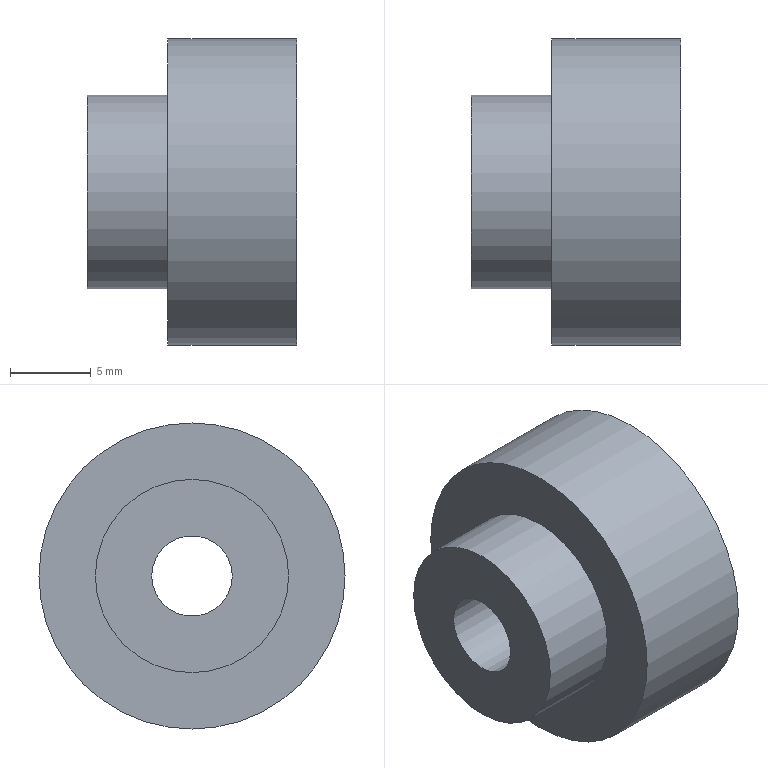Part | STEP file | 1-46.3 | 1 solid | 6 faces | box 13 x 19 x 19 mm | volume 2578 mm3 | plane 3 | cylinder 3 | commonest cylinder face diameters 5 x1 12 x1 19 x1
STEP:
#1=CARTESIAN_POINT('',(0.,0.,0.));
#2=DIRECTION('',(0.,0.,1.));
#3=DIRECTION('',(1.,0.,0.));
#4=AXIS2_PLACEMENT_3D('',#1,#2,#3);
#5=CARTESIAN_POINT('',(-5.,6.,0.));
#6=VERTEX_POINT('',#5);
#7=CARTESIAN_POINT('',(-5.,0.,0.));
#8=DIRECTION('',(1.,0.,0.));
#9=DIRECTION('',(0.,1.,0.));
#10=AXIS2_PLACEMENT_3D('',#7,#8,#9);
#11=CIRCLE('',#10,6.);
#12=CARTESIAN_POINT('',(-5.,-1.608,0.));
#13=DIRECTION('',(1.,0.,0.));
#14=DIRECTION('',(0.,0.,-1.));
#15=AXIS2_PLACEMENT_3D('',#12,#13,#14);
#16=PLANE('',#15);
#17=CARTESIAN_POINT('',(0.,1.608));
#18=DIRECTION('',(0.,1.));
#19=AXIS2_PLACEMENT_2D('',#17,#18);
#20=CIRCLE('',#19,6.);
#21=(GEOMETRIC_REPRESENTATION_CONTEXT(2)PARAMETRIC_REPRESENTATION_CONTEXT()REPRESENTATION_CONTEXT('',''));
#22=DEFINITIONAL_REPRESENTATION('',(#20),#21);
#23=PCURVE('',#16,#22);
#24=CARTESIAN_POINT('',(0.,0.,0.));
#25=DIRECTION('',(-1.,0.,0.));
#26=DIRECTION('',(0.,1.,0.));
#27=AXIS2_PLACEMENT_3D('',#24,#25,#26);
#28=CYLINDRICAL_SURFACE('',#27,6.);
#29=CARTESIAN_POINT('',(6.283,5.));
#30=DIRECTION('',(-1.,0.));
#31=VECTOR('',#30,1.);
#32=LINE('',#29,#31);
#33=(GEOMETRIC_REPRESENTATION_CONTEXT(2)PARAMETRIC_REPRESENTATION_CONTEXT()REPRESENTATION_CONTEXT('',''));
#34=DEFINITIONAL_REPRESENTATION('',(#32),#33);
#35=PCURVE('',#28,#34);
#36=SURFACE_CURVE('',#11,(#23,#35),.PCURVE_S1.);
#37=EDGE_CURVE('',#6,#6,#36,.T.);
#38=ORIENTED_EDGE('',*,*,#37,.T.);
#39=EDGE_LOOP('',(#38));
#40=FACE_BOUND('',#39,.F.);
#41=CARTESIAN_POINT('',(-5.,2.5,0.));
#42=VERTEX_POINT('',#41);
#43=CARTESIAN_POINT('',(-5.,0.,0.));
#44=DIRECTION('',(-1.,0.,0.));
#45=DIRECTION('',(0.,1.,0.));
#46=AXIS2_PLACEMENT_3D('',#43,#44,#45);
#47=CIRCLE('',#46,2.5);
#48=CARTESIAN_POINT('',(0.,4.108));
#49=CARTESIAN_POINT('',(4.33,4.108));
#50=CARTESIAN_POINT('',(2.165,0.3577));
#51=CARTESIAN_POINT('',(0.,-3.392));
#52=CARTESIAN_POINT('',(-2.165,0.3577));
#53=CARTESIAN_POINT('',(-4.33,4.108));
#54=CARTESIAN_POINT('',(0.,4.108));
#55=(BOUNDED_CURVE()B_SPLINE_CURVE(2,(#48,#49,#50,#51,#52,#53,#54),.UNSPECIFIED.,.T.,.F.)B_SPLINE_CURVE_WITH_KNOTS((1,2,2,2,2,1),(-2.094,0.,2.094,4.189,6.283,8.378),.UNSPECIFIED.)CURVE()GEOMETRIC_REPRESENTATION_ITEM()RATIONAL_B_SPLINE_CURVE((1.,0.5,1.,0.5,1.,0.5,1.))REPRESENTATION_ITEM(''));
#56=(GEOMETRIC_REPRESENTATION_CONTEXT(2)PARAMETRIC_REPRESENTATION_CONTEXT()REPRESENTATION_CONTEXT('',''));
#57=DEFINITIONAL_REPRESENTATION('',(#55),#56);
#58=PCURVE('',#16,#57);
#59=CARTESIAN_POINT('',(8.,0.,0.));
#60=DIRECTION('',(-1.,0.,0.));
#61=DIRECTION('',(0.,1.,0.));
#62=AXIS2_PLACEMENT_3D('',#59,#60,#61);
#63=CYLINDRICAL_SURFACE('',#62,2.5);
#64=CARTESIAN_POINT('',(0.,13.));
#65=DIRECTION('',(1.,0.));
#66=VECTOR('',#65,1.);
#67=LINE('',#64,#66);
#68=(GEOMETRIC_REPRESENTATION_CONTEXT(2)PARAMETRIC_REPRESENTATION_CONTEXT()REPRESENTATION_CONTEXT('',''));
#69=DEFINITIONAL_REPRESENTATION('',(#67),#68);
#70=PCURVE('',#63,#69);
#71=SURFACE_CURVE('',#47,(#58,#70),.PCURVE_S1.);
#72=EDGE_CURVE('',#42,#42,#71,.T.);
#73=ORIENTED_EDGE('',*,*,#72,.T.);
#74=EDGE_LOOP('',(#73));
#75=FACE_BOUND('',#74,.F.);
#76=ADVANCED_FACE('',(#40,#75),#16,.F.);
#77=CARTESIAN_POINT('',(0.,6.,0.));
#78=VERTEX_POINT('',#77);
#79=CARTESIAN_POINT('',(0.,6.,0.));
#80=DIRECTION('',(-1.,0.,0.));
#81=VECTOR('',#80,1.);
#82=LINE('',#79,#81);
#83=CARTESIAN_POINT('',(6.283,0.));
#84=DIRECTION('',(0.,1.));
#85=VECTOR('',#84,1.);
#86=LINE('',#83,#85);
#87=(GEOMETRIC_REPRESENTATION_CONTEXT(2)PARAMETRIC_REPRESENTATION_CONTEXT()REPRESENTATION_CONTEXT('',''));
#88=DEFINITIONAL_REPRESENTATION('',(#86),#87);
#89=PCURVE('',#28,#88);
#90=CARTESIAN_POINT('',(0.,0.));
#91=DIRECTION('',(0.,1.));
#92=VECTOR('',#91,1.);
#93=LINE('',#90,#92);
#94=(GEOMETRIC_REPRESENTATION_CONTEXT(2)PARAMETRIC_REPRESENTATION_CONTEXT()REPRESENTATION_CONTEXT('',''));
#95=DEFINITIONAL_REPRESENTATION('',(#93),#94);
#96=PCURVE('',#28,#95);
#97=SEAM_CURVE('',#82,(#89,#96),.PCURVE_S1.);
#98=EDGE_CURVE('',#78,#6,#97,.T.);
#99=ORIENTED_EDGE('',*,*,#98,.T.);
#100=ORIENTED_EDGE('',*,*,#37,.T.);
#101=ORIENTED_EDGE('',*,*,#98,.F.);
#102=CARTESIAN_POINT('',(0.,0.,0.));
#103=DIRECTION('',(1.,0.,0.));
#104=DIRECTION('',(0.,1.,0.));
#105=AXIS2_PLACEMENT_3D('',#102,#103,#104);
#106=CIRCLE('',#105,6.);
#107=CARTESIAN_POINT('',(6.283,0.));
#108=DIRECTION('',(-1.,0.));
#109=VECTOR('',#108,1.);
#110=LINE('',#107,#109);
#111=(GEOMETRIC_REPRESENTATION_CONTEXT(2)PARAMETRIC_REPRESENTATION_CONTEXT()REPRESENTATION_CONTEXT('',''));
#112=DEFINITIONAL_REPRESENTATION('',(#110),#111);
#113=PCURVE('',#28,#112);
#114=CARTESIAN_POINT('',(0.,-2.546,0.));
#115=DIRECTION('',(1.,0.,0.));
#116=DIRECTION('',(0.,0.,-1.));
#117=AXIS2_PLACEMENT_3D('',#114,#115,#116);
#118=PLANE('',#117);
#119=CARTESIAN_POINT('',(0.,2.546));
#120=DIRECTION('',(0.,1.));
#121=AXIS2_PLACEMENT_2D('',#119,#120);
#122=CIRCLE('',#121,6.);
#123=(GEOMETRIC_REPRESENTATION_CONTEXT(2)PARAMETRIC_REPRESENTATION_CONTEXT()REPRESENTATION_CONTEXT('',''));
#124=DEFINITIONAL_REPRESENTATION('',(#122),#123);
#125=PCURVE('',#118,#124);
#126=SURFACE_CURVE('',#106,(#113,#125),.PCURVE_S1.);
#127=EDGE_CURVE('',#78,#78,#126,.T.);
#128=ORIENTED_EDGE('',*,*,#127,.F.);
#129=EDGE_LOOP('',(#99,#100,#101,#128));
#130=FACE_BOUND('',#129,.T.);
#131=ADVANCED_FACE('',(#130),#28,.T.);
#132=ORIENTED_EDGE('',*,*,#72,.F.);
#133=CARTESIAN_POINT('',(8.,2.5,0.));
#134=VERTEX_POINT('',#133);
#135=CARTESIAN_POINT('',(-5.,2.5,0.));
#136=DIRECTION('',(1.,0.,0.));
#137=VECTOR('',#136,1.);
#138=LINE('',#135,#137);
#139=CARTESIAN_POINT('',(0.,13.));
#140=DIRECTION('',(0.,-1.));
#141=VECTOR('',#140,1.);
#142=LINE('',#139,#141);
#143=(GEOMETRIC_REPRESENTATION_CONTEXT(2)PARAMETRIC_REPRESENTATION_CONTEXT()REPRESENTATION_CONTEXT('',''));
#144=DEFINITIONAL_REPRESENTATION('',(#142),#143);
#145=PCURVE('',#63,#144);
#146=CARTESIAN_POINT('',(6.283,13.));
#147=DIRECTION('',(0.,-1.));
#148=VECTOR('',#147,1.);
#149=LINE('',#146,#148);
#150=(GEOMETRIC_REPRESENTATION_CONTEXT(2)PARAMETRIC_REPRESENTATION_CONTEXT()REPRESENTATION_CONTEXT('',''));
#151=DEFINITIONAL_REPRESENTATION('',(#149),#150);
#152=PCURVE('',#63,#151);
#153=SEAM_CURVE('',#138,(#145,#152),.PCURVE_S1.);
#154=EDGE_CURVE('',#42,#134,#153,.T.);
#155=ORIENTED_EDGE('',*,*,#154,.T.);
#156=CARTESIAN_POINT('',(8.,0.,0.));
#157=DIRECTION('',(-1.,0.,0.));
#158=DIRECTION('',(0.,1.,0.));
#159=AXIS2_PLACEMENT_3D('',#156,#157,#158);
#160=CIRCLE('',#159,2.5);
#161=CARTESIAN_POINT('',(0.,0.));
#162=DIRECTION('',(1.,0.));
#163=VECTOR('',#162,1.);
#164=LINE('',#161,#163);
#165=(GEOMETRIC_REPRESENTATION_CONTEXT(2)PARAMETRIC_REPRESENTATION_CONTEXT()REPRESENTATION_CONTEXT('',''));
#166=DEFINITIONAL_REPRESENTATION('',(#164),#165);
#167=PCURVE('',#63,#166);
#168=CARTESIAN_POINT('',(8.,-2.546,0.));
#169=DIRECTION('',(1.,0.,0.));
#170=DIRECTION('',(0.,0.,-1.));
#171=AXIS2_PLACEMENT_3D('',#168,#169,#170);
#172=PLANE('',#171);
#173=CARTESIAN_POINT('',(0.,5.046));
#174=CARTESIAN_POINT('',(4.33,5.046));
#175=CARTESIAN_POINT('',(2.165,1.296));
#176=CARTESIAN_POINT('',(0.,-2.454));
#177=CARTESIAN_POINT('',(-2.165,1.296));
#178=CARTESIAN_POINT('',(-4.33,5.046));
#179=CARTESIAN_POINT('',(0.,5.046));
#180=(BOUNDED_CURVE()B_SPLINE_CURVE(2,(#173,#174,#175,#176,#177,#178,#179),.UNSPECIFIED.,.T.,.F.)B_SPLINE_CURVE_WITH_KNOTS((1,2,2,2,2,1),(-2.094,0.,2.094,4.189,6.283,8.378),.UNSPECIFIED.)CURVE()GEOMETRIC_REPRESENTATION_ITEM()RATIONAL_B_SPLINE_CURVE((1.,0.5,1.,0.5,1.,0.5,1.))REPRESENTATION_ITEM(''));
#181=(GEOMETRIC_REPRESENTATION_CONTEXT(2)PARAMETRIC_REPRESENTATION_CONTEXT()REPRESENTATION_CONTEXT('',''));
#182=DEFINITIONAL_REPRESENTATION('',(#180),#181);
#183=PCURVE('',#172,#182);
#184=SURFACE_CURVE('',#160,(#167,#183),.PCURVE_S1.);
#185=EDGE_CURVE('',#134,#134,#184,.T.);
#186=ORIENTED_EDGE('',*,*,#185,.T.);
#187=ORIENTED_EDGE('',*,*,#154,.F.);
#188=EDGE_LOOP('',(#132,#155,#186,#187));
#189=FACE_BOUND('',#188,.F.);
#190=ADVANCED_FACE('',(#189),#63,.F.);
#191=CARTESIAN_POINT('',(0.,9.5,0.));
#192=VERTEX_POINT('',#191);
#193=CARTESIAN_POINT('',(0.,0.,0.));
#194=DIRECTION('',(1.,0.,0.));
#195=DIRECTION('',(0.,1.,0.));
#196=AXIS2_PLACEMENT_3D('',#193,#194,#195);
#197=CIRCLE('',#196,9.5);
#198=CARTESIAN_POINT('',(0.,2.546));
#199=DIRECTION('',(0.,1.));
#200=AXIS2_PLACEMENT_2D('',#198,#199);
#201=CIRCLE('',#200,9.5);
#202=(GEOMETRIC_REPRESENTATION_CONTEXT(2)PARAMETRIC_REPRESENTATION_CONTEXT()REPRESENTATION_CONTEXT('',''));
#203=DEFINITIONAL_REPRESENTATION('',(#201),#202);
#204=PCURVE('',#118,#203);
#205=CARTESIAN_POINT('',(0.,0.,0.));
#206=DIRECTION('',(1.,0.,0.));
#207=DIRECTION('',(0.,1.,0.));
#208=AXIS2_PLACEMENT_3D('',#205,#206,#207);
#209=CYLINDRICAL_SURFACE('',#208,9.5);
#210=CARTESIAN_POINT('',(0.,0.));
#211=DIRECTION('',(1.,0.));
#212=VECTOR('',#211,1.);
#213=LINE('',#210,#212);
#214=(GEOMETRIC_REPRESENTATION_CONTEXT(2)PARAMETRIC_REPRESENTATION_CONTEXT()REPRESENTATION_CONTEXT('',''));
#215=DEFINITIONAL_REPRESENTATION('',(#213),#214);
#216=PCURVE('',#209,#215);
#217=SURFACE_CURVE('',#197,(#204,#216),.PCURVE_S1.);
#218=EDGE_CURVE('',#192,#192,#217,.T.);
#219=ORIENTED_EDGE('',*,*,#218,.T.);
#220=EDGE_LOOP('',(#219));
#221=FACE_BOUND('',#220,.F.);
#222=ORIENTED_EDGE('',*,*,#127,.F.);
#223=EDGE_LOOP('',(#222));
#224=FACE_BOUND('',#223,.F.);
#225=ADVANCED_FACE('',(#221,#224),#118,.F.);
#226=ORIENTED_EDGE('',*,*,#218,.T.);
#227=CARTESIAN_POINT('',(8.,9.5,0.));
#228=VERTEX_POINT('',#227);
#229=CARTESIAN_POINT('',(0.,9.5,0.));
#230=DIRECTION('',(1.,0.,0.));
#231=VECTOR('',#230,1.);
#232=LINE('',#229,#231);
#233=CARTESIAN_POINT('',(6.283,0.));
#234=DIRECTION('',(0.,1.));
#235=VECTOR('',#234,1.);
#236=LINE('',#233,#235);
#237=(GEOMETRIC_REPRESENTATION_CONTEXT(2)PARAMETRIC_REPRESENTATION_CONTEXT()REPRESENTATION_CONTEXT('',''));
#238=DEFINITIONAL_REPRESENTATION('',(#236),#237);
#239=PCURVE('',#209,#238);
#240=CARTESIAN_POINT('',(0.,0.));
#241=DIRECTION('',(0.,1.));
#242=VECTOR('',#241,1.);
#243=LINE('',#240,#242);
#244=(GEOMETRIC_REPRESENTATION_CONTEXT(2)PARAMETRIC_REPRESENTATION_CONTEXT()REPRESENTATION_CONTEXT('',''));
#245=DEFINITIONAL_REPRESENTATION('',(#243),#244);
#246=PCURVE('',#209,#245);
#247=SEAM_CURVE('',#232,(#239,#246),.PCURVE_S1.);
#248=EDGE_CURVE('',#192,#228,#247,.T.);
#249=ORIENTED_EDGE('',*,*,#248,.T.);
#250=CARTESIAN_POINT('',(8.,0.,0.));
#251=DIRECTION('',(1.,0.,0.));
#252=DIRECTION('',(0.,1.,0.));
#253=AXIS2_PLACEMENT_3D('',#250,#251,#252);
#254=CIRCLE('',#253,9.5);
#255=CARTESIAN_POINT('',(0.,8.));
#256=DIRECTION('',(1.,0.));
#257=VECTOR('',#256,1.);
#258=LINE('',#255,#257);
#259=(GEOMETRIC_REPRESENTATION_CONTEXT(2)PARAMETRIC_REPRESENTATION_CONTEXT()REPRESENTATION_CONTEXT('',''));
#260=DEFINITIONAL_REPRESENTATION('',(#258),#259);
#261=PCURVE('',#209,#260);
#262=CARTESIAN_POINT('',(0.,2.546));
#263=DIRECTION('',(0.,1.));
#264=AXIS2_PLACEMENT_2D('',#262,#263);
#265=CIRCLE('',#264,9.5);
#266=(GEOMETRIC_REPRESENTATION_CONTEXT(2)PARAMETRIC_REPRESENTATION_CONTEXT()REPRESENTATION_CONTEXT('',''));
#267=DEFINITIONAL_REPRESENTATION('',(#265),#266);
#268=PCURVE('',#172,#267);
#269=SURFACE_CURVE('',#254,(#261,#268),.PCURVE_S1.);
#270=EDGE_CURVE('',#228,#228,#269,.T.);
#271=ORIENTED_EDGE('',*,*,#270,.F.);
#272=ORIENTED_EDGE('',*,*,#248,.F.);
#273=EDGE_LOOP('',(#226,#249,#271,#272));
#274=FACE_BOUND('',#273,.T.);
#275=ADVANCED_FACE('',(#274),#209,.T.);
#276=ORIENTED_EDGE('',*,*,#270,.T.);
#277=EDGE_LOOP('',(#276));
#278=FACE_BOUND('',#277,.T.);
#279=ORIENTED_EDGE('',*,*,#185,.T.);
#280=EDGE_LOOP('',(#279));
#281=FACE_BOUND('',#280,.T.);
#282=ADVANCED_FACE('',(#278,#281),#172,.T.);
#283=CLOSED_SHELL('',(#76,#131,#190,#225,#275,#282));
#284=MANIFOLD_SOLID_BREP('',#283);
#285=(LENGTH_UNIT()NAMED_UNIT(*)SI_UNIT(.MILLI.,.METRE.));
#286=UNCERTAINTY_MEASURE_WITH_UNIT(LENGTH_MEASURE(0.0000001),#285,'','');
#287=(NAMED_UNIT(*)PLANE_ANGLE_UNIT()SI_UNIT($,.RADIAN.));
#288=(NAMED_UNIT(*)SI_UNIT($,.STERADIAN.)SOLID_ANGLE_UNIT());
#289=(GEOMETRIC_REPRESENTATION_CONTEXT(3)GLOBAL_UNCERTAINTY_ASSIGNED_CONTEXT((#286))GLOBAL_UNIT_ASSIGNED_CONTEXT((#285,#287,#288))REPRESENTATION_CONTEXT('',''));
#290=ADVANCED_BREP_SHAPE_REPRESENTATION('',(#4,#284),#289);